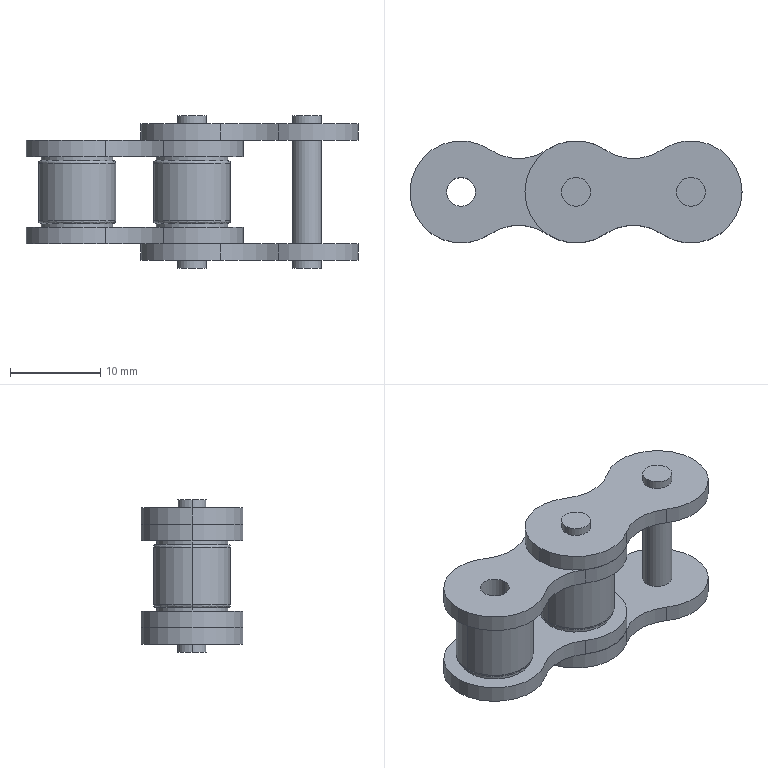Part | STEP file | 08b1v1V11 | 1 solid | 68 faces | box 36.689 x 11.289 x 16.9 mm | volume 2497 mm3 | cylinder 48 | plane 12 | spline 8 | commonest cylinder face diameters 11.289 x20 3.191 x16 7.91 x8 8.51 x4